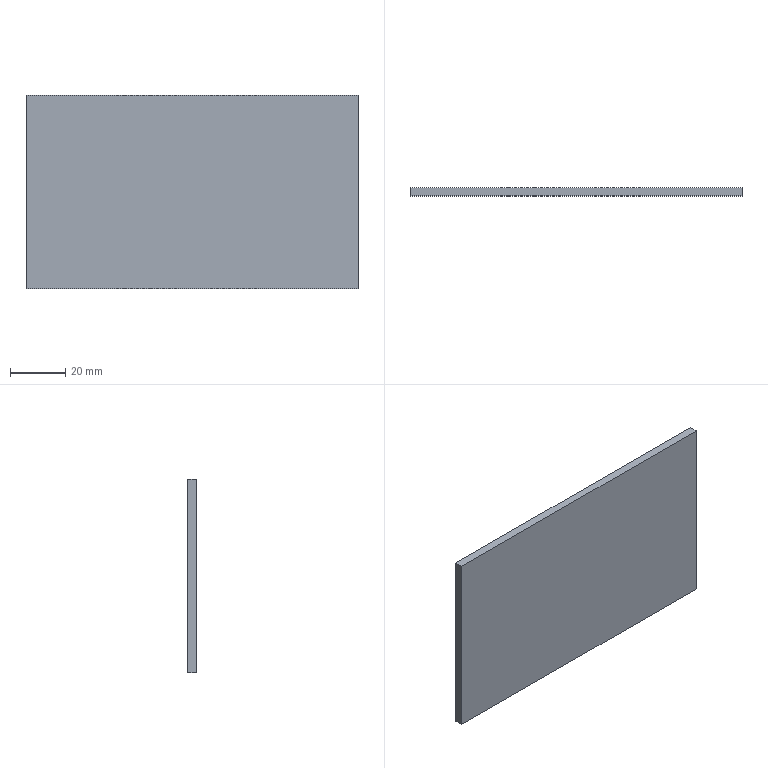Part | SolidWorks | features Extrusion 1 | 1 solid | 6 faces | box 120 x 3 x 70 mm | volume 25200 mm3 | plane 6
STEP:
#1=CARTESIAN_POINT('',(-60.,1.5,0.));
#2=VERTEX_POINT('',#1);
#3=CARTESIAN_POINT('',(-60.,-1.5,0.));
#4=VERTEX_POINT('',#3);
#5=CARTESIAN_POINT('',(-60.,-1.5,0.));
#6=DIRECTION('',(0.,-1.,0.));
#7=VECTOR('',#6,1000.);
#8=LINE('',#5,#7);
#9=EDGE_CURVE('',#2,#4,#8,.T.);
#10=ORIENTED_EDGE('',*,*,#9,.T.);
#11=CARTESIAN_POINT('',(-60.,-1.5,70.));
#12=VERTEX_POINT('',#11);
#13=CARTESIAN_POINT('',(-60.,-1.5,70.));
#14=DIRECTION('',(0.,0.,-1.));
#15=VECTOR('',#14,1000.);
#16=LINE('',#13,#15);
#17=EDGE_CURVE('',#12,#4,#16,.T.);
#18=ORIENTED_EDGE('',*,*,#17,.F.);
#19=CARTESIAN_POINT('',(-60.,1.5,70.));
#20=VERTEX_POINT('',#19);
#21=CARTESIAN_POINT('',(-60.,-1.5,70.));
#22=DIRECTION('',(0.,-1.,0.));
#23=VECTOR('',#22,1000.);
#24=LINE('',#21,#23);
#25=EDGE_CURVE('',#20,#12,#24,.T.);
#26=ORIENTED_EDGE('',*,*,#25,.F.);
#27=CARTESIAN_POINT('',(-60.,1.5,70.));
#28=DIRECTION('',(0.,0.,-1.));
#29=VECTOR('',#28,1000.);
#30=LINE('',#27,#29);
#31=EDGE_CURVE('',#20,#2,#30,.T.);
#32=ORIENTED_EDGE('',*,*,#31,.T.);
#33=EDGE_LOOP('',(#10,#18,#26,#32));
#34=FACE_OUTER_BOUND('',#33,.T.);
#35=CARTESIAN_POINT('',(-60.,-1.5,70.));
#36=DIRECTION('',(1.,0.,0.));
#37=DIRECTION('',(0.,0.,-1.));
#38=AXIS2_PLACEMENT_3D('',#35,#36,#37);
#39=PLANE('',#38);
#40=ADVANCED_FACE('',(#34),#39,.F.);
#41=CARTESIAN_POINT('',(60.,-1.5,0.));
#42=VERTEX_POINT('',#41);
#43=CARTESIAN_POINT('',(60.,-1.5,0.));
#44=DIRECTION('',(1.,0.,0.));
#45=VECTOR('',#44,1000.);
#46=LINE('',#43,#45);
#47=EDGE_CURVE('',#4,#42,#46,.T.);
#48=ORIENTED_EDGE('',*,*,#47,.T.);
#49=CARTESIAN_POINT('',(60.,-1.5,70.));
#50=VERTEX_POINT('',#49);
#51=CARTESIAN_POINT('',(60.,-1.5,70.));
#52=DIRECTION('',(0.,0.,-1.));
#53=VECTOR('',#52,1000.);
#54=LINE('',#51,#53);
#55=EDGE_CURVE('',#50,#42,#54,.T.);
#56=ORIENTED_EDGE('',*,*,#55,.F.);
#57=CARTESIAN_POINT('',(60.,-1.5,70.));
#58=DIRECTION('',(1.,0.,0.));
#59=VECTOR('',#58,1000.);
#60=LINE('',#57,#59);
#61=EDGE_CURVE('',#12,#50,#60,.T.);
#62=ORIENTED_EDGE('',*,*,#61,.F.);
#63=ORIENTED_EDGE('',*,*,#17,.T.);
#64=EDGE_LOOP('',(#48,#56,#62,#63));
#65=FACE_OUTER_BOUND('',#64,.T.);
#66=CARTESIAN_POINT('',(60.,-1.5,70.));
#67=DIRECTION('',(0.,1.,0.));
#68=DIRECTION('',(-1.,0.,0.));
#69=AXIS2_PLACEMENT_3D('',#66,#67,#68);
#70=PLANE('',#69);
#71=ADVANCED_FACE('',(#65),#70,.F.);
#72=CARTESIAN_POINT('',(60.,1.5,0.));
#73=VERTEX_POINT('',#72);
#74=CARTESIAN_POINT('',(60.,-1.5,0.));
#75=DIRECTION('',(0.,1.,0.));
#76=VECTOR('',#75,1000.);
#77=LINE('',#74,#76);
#78=EDGE_CURVE('',#42,#73,#77,.T.);
#79=ORIENTED_EDGE('',*,*,#78,.T.);
#80=CARTESIAN_POINT('',(60.,1.5,70.));
#81=VERTEX_POINT('',#80);
#82=CARTESIAN_POINT('',(60.,1.5,70.));
#83=DIRECTION('',(0.,0.,-1.));
#84=VECTOR('',#83,1000.);
#85=LINE('',#82,#84);
#86=EDGE_CURVE('',#81,#73,#85,.T.);
#87=ORIENTED_EDGE('',*,*,#86,.F.);
#88=CARTESIAN_POINT('',(60.,-1.5,70.));
#89=DIRECTION('',(0.,1.,0.));
#90=VECTOR('',#89,1000.);
#91=LINE('',#88,#90);
#92=EDGE_CURVE('',#50,#81,#91,.T.);
#93=ORIENTED_EDGE('',*,*,#92,.F.);
#94=ORIENTED_EDGE('',*,*,#55,.T.);
#95=EDGE_LOOP('',(#79,#87,#93,#94));
#96=FACE_OUTER_BOUND('',#95,.T.);
#97=CARTESIAN_POINT('',(60.,-1.5,70.));
#98=DIRECTION('',(-1.,0.,0.));
#99=DIRECTION('',(0.,0.,1.));
#100=AXIS2_PLACEMENT_3D('',#97,#98,#99);
#101=PLANE('',#100);
#102=ADVANCED_FACE('',(#96),#101,.F.);
#103=CARTESIAN_POINT('',(60.,1.5,0.));
#104=DIRECTION('',(-1.,0.,0.));
#105=VECTOR('',#104,1000.);
#106=LINE('',#103,#105);
#107=EDGE_CURVE('',#73,#2,#106,.T.);
#108=ORIENTED_EDGE('',*,*,#107,.T.);
#109=ORIENTED_EDGE('',*,*,#31,.F.);
#110=CARTESIAN_POINT('',(60.,1.5,70.));
#111=DIRECTION('',(-1.,0.,0.));
#112=VECTOR('',#111,1000.);
#113=LINE('',#110,#112);
#114=EDGE_CURVE('',#81,#20,#113,.T.);
#115=ORIENTED_EDGE('',*,*,#114,.F.);
#116=ORIENTED_EDGE('',*,*,#86,.T.);
#117=EDGE_LOOP('',(#108,#109,#115,#116));
#118=FACE_OUTER_BOUND('',#117,.T.);
#119=CARTESIAN_POINT('',(60.,1.5,70.));
#120=DIRECTION('',(0.,-1.,0.));
#121=DIRECTION('',(1.,0.,0.));
#122=AXIS2_PLACEMENT_3D('',#119,#120,#121);
#123=PLANE('',#122);
#124=ADVANCED_FACE('',(#118),#123,.F.);
#125=ORIENTED_EDGE('',*,*,#25,.T.);
#126=ORIENTED_EDGE('',*,*,#61,.T.);
#127=ORIENTED_EDGE('',*,*,#92,.T.);
#128=ORIENTED_EDGE('',*,*,#114,.T.);
#129=EDGE_LOOP('',(#125,#126,#127,#128));
#130=FACE_OUTER_BOUND('',#129,.T.);
#131=CARTESIAN_POINT('',(0.,0.,70.));
#132=DIRECTION('',(0.,0.,1.));
#133=DIRECTION('',(1.,0.,0.));
#134=AXIS2_PLACEMENT_3D('',#131,#132,#133);
#135=PLANE('',#134);
#136=ADVANCED_FACE('',(#130),#135,.T.);
#137=ORIENTED_EDGE('',*,*,#9,.F.);
#138=ORIENTED_EDGE('',*,*,#107,.F.);
#139=ORIENTED_EDGE('',*,*,#78,.F.);
#140=ORIENTED_EDGE('',*,*,#47,.F.);
#141=EDGE_LOOP('',(#137,#138,#139,#140));
#142=FACE_OUTER_BOUND('',#141,.T.);
#143=CARTESIAN_POINT('',(0.,0.,0.));
#144=DIRECTION('',(0.,0.,1.));
#145=DIRECTION('',(1.,0.,0.));
#146=AXIS2_PLACEMENT_3D('',#143,#144,#145);
#147=PLANE('',#146);
#148=ADVANCED_FACE('',(#142),#147,.F.);
#149=CLOSED_SHELL('',(#40,#71,#102,#124,#136,#148));
#150=MANIFOLD_SOLID_BREP('',#149);
#151=CARTESIAN_POINT('',(0.,0.,0.));
#152=DIRECTION('',(0.,0.,1.));
#153=DIRECTION('',(1.,0.,0.));
#154=AXIS2_PLACEMENT_3D('',#151,#152,#153);
#155=(LENGTH_UNIT()NAMED_UNIT(*)SI_UNIT(.MILLI.,.METRE.));
#156=UNCERTAINTY_MEASURE_WITH_UNIT(LENGTH_MEASURE(0.00001),#155,'','');
#157=(NAMED_UNIT(*)PLANE_ANGLE_UNIT()SI_UNIT($,.RADIAN.));
#158=(NAMED_UNIT(*)SI_UNIT($,.STERADIAN.)SOLID_ANGLE_UNIT());
#159=(GEOMETRIC_REPRESENTATION_CONTEXT(3)GLOBAL_UNCERTAINTY_ASSIGNED_CONTEXT((#156))GLOBAL_UNIT_ASSIGNED_CONTEXT((#155,#157,#158))REPRESENTATION_CONTEXT('',''));
#160=ADVANCED_BREP_SHAPE_REPRESENTATION('',(#150,#154),#159);